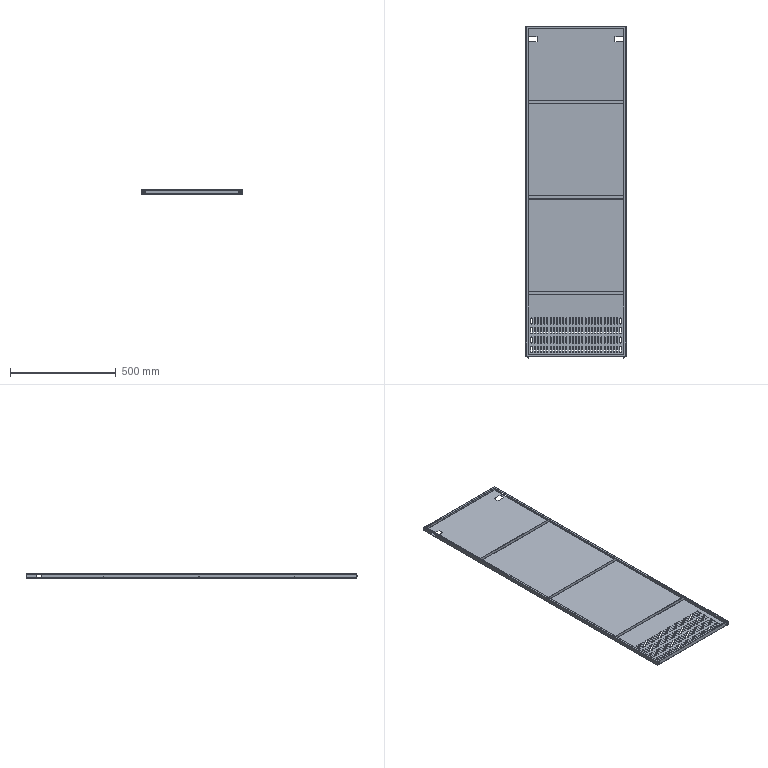Part | SolidWorks | features CompositeCurve 2 | 7 solids | 646 faces | box 473 x 1568 x 20 mm | volume 883759 mm3 | plane 340 | cylinder 274 | spline 16 | torus 16 | commonest cylinder face diameters 5 x232 0.2 x14 2.2 x12 4 x8 4.5 x4 8 x4